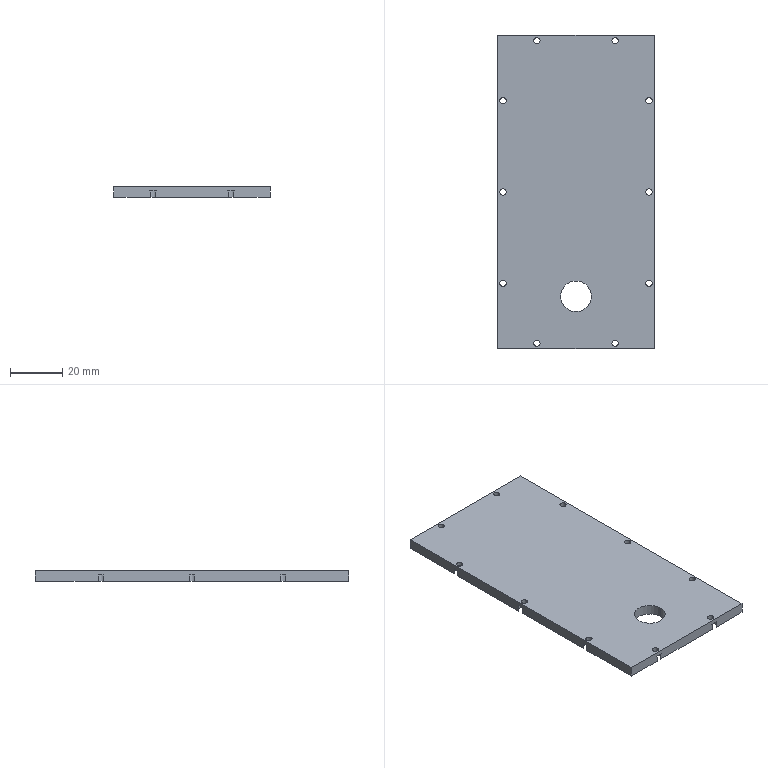Part | SolidWorks | features Extrusion 1, HoleWzd 1, ICE 1 | 1 solid | 59 faces | box 60 x 120 x 4 mm | volume 27931 mm3 | cylinder 43 | plane 16 | commonest cylinder face diameters 4.4 x21 2.4 x20 11.8 x2